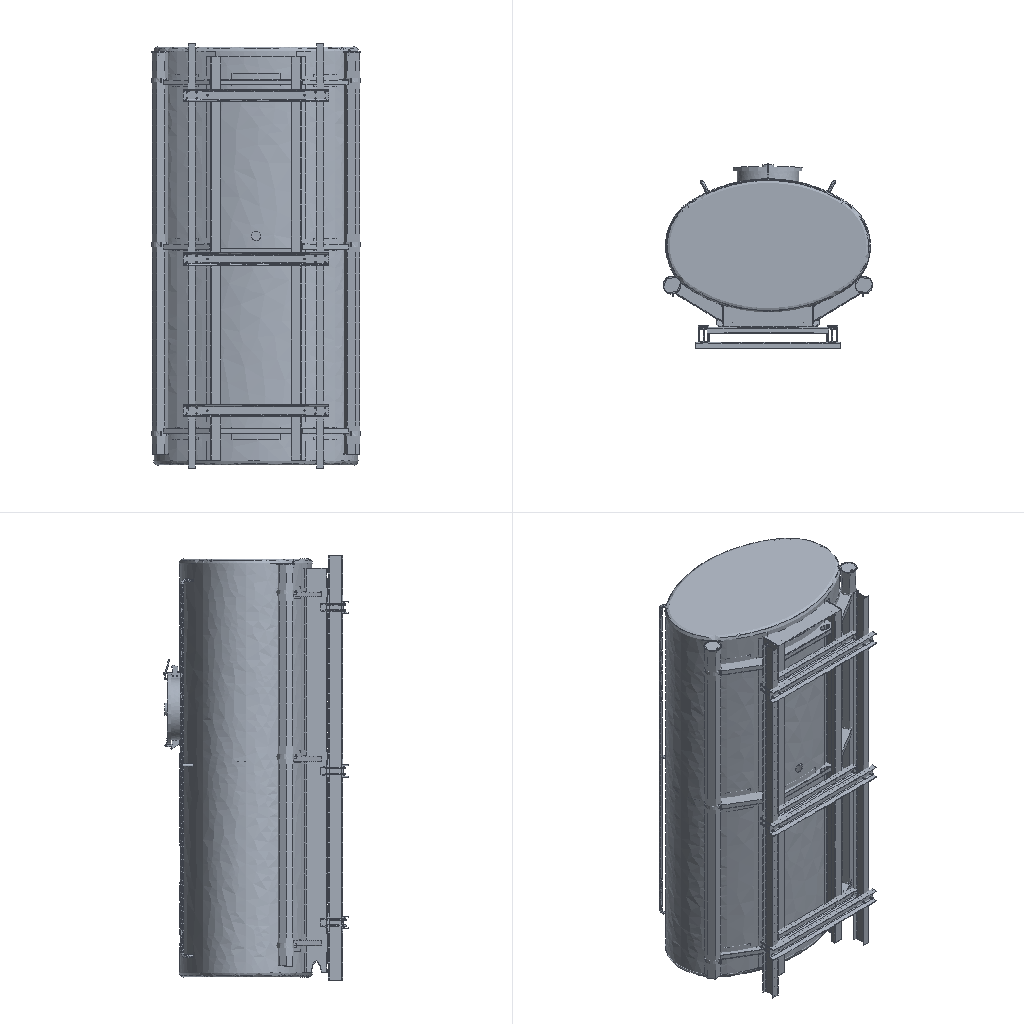Simulation study | ansys workbench
Ansys APDL input file, long lists of numbers shortened:
/batch
/config,noeldb,1     ! force off writing results to database
*get,_wallstrt,active,,time,wall
! ANSYS input file written by Workbench version 2022 R1
! File used for geometry attach: F:\ansys（分析文件汇总)\洒水车有限元分析\晒水车罐体.STEP
/title,wbnew--____ (D5)
! ****** Begin Custom Load Command Snippet ******
/COM, ACT Extensions:
/COM,     LSDYNA, 2021.1
/COM,
! ****** End   Custom Load Command Snippet ******
*DIM,_wb_ProjectScratch_dir,string,248
_wb_ProjectScratch_dir(1) = 'C:\Users\Administrator\AppData\Local\Temp\WB_Administrator_19044_2\_ProjectScratch\ScrCD54\'
*DIM,_wb_SolverFiles_dir,string,248
_wb_SolverFiles_dir(1) = 'C:\Users\Administrator\AppData\Local\Temp\WB_Administrator_19044_2\wbnew_files\dp0\SYS-2\MECH\'
*DIM,_wb_userfiles_dir,string,248
_wb_userfiles_dir(1) = 'C:\Users\Administrator\AppData\Local\Temp\WB_Administrator_19044_2\wbnew_files\user_files\'
/com,--- Data in consistent NMM units. See Solving Units in the help system for more information.
/units,MPA
/nopr
/wb,file,start              !  signify a WB generated input file
/prep7
! Turn off shape checking because checks already performed inside WB mesher.
! See help system for more information.
SHPP,OFF,,NOWARN
/nolist
etcon,set             ! allow ANSYS to choose best KEYOP's for 180x elements, resets any applicable keyopt to MAPDL defaults
/com,*********** Nodes for the whole assembly ***********
nblock,3,,154514
(1i9,3e20.9e3)
    59613    -4.978285790E+02     4.306437121E+02     3.184288870E+01
! (140467 more lines like these left out)
-1
/wb,elem,start            !  set before creation of elements
/com,*********** Elements for Body 1 "__|1210-011-G03|__-__1" ***********
et,1,187
eblock,19,solid,,5134
(19i9)
        1        1        1        1        0        0        0        0       10        0        1     1367     1730     1457     1374     9329     9682     9325     9324
! (10267 more lines like these left out)
-1
/com,*********** Elements for Body 2 "__|1210-011-G03|__-__1[2]" ***********
et,2,187
eblock,19,solid,,5134
(19i9)
        2        2        2        2        0        0        0        0       10        0     5135    12093    12456    12183    12100    20055    20408    20051    20050
! (10267 more lines like these left out)
-1
/com,*********** Elements for Body 3 "__|__-0|__-__3" ***********
et,3,187
eblock,19,solid,,12299
(19i9)
        3        3        3        3        0        0        0        0       10        0    10269    22599    23787    23678    22852    33647    40850    33645    33640
! (24597 more lines like these left out)
-1
/com,*********** Elements for Body 4 "__|1210-041-G03|__-__9" ***********
et,4,187
eblock,19,solid,,1630
(19i9)
        4        4        4        4        0        0        0        0       10        0    22568    46545    47052    46995    46688    47336    49436    47333    47330
! (3259 more lines like these left out)
-1
/com,*********** Elements for Body 5 "__|1210-042-G03|__-__1" ***********
et,5,186
keyo,5,2,1          ! set full integration on SOLID186
eblock,19,solid,,62
(19i9)
        5        5        5        5        0        0        0        0       20        0    24198    50489    50500    50499    50490    50548    50537    50538    50539
! (123 more lines like these left out)
-1
! (74 more sections like these left out)
/wb,elem,end               !  done creating elements
/com,*********** Send User Defined Coordinate System(s) ***********
csys,0
toffst,273.15,  ! Temperature offset from absolute zero
/com,*********** Set Reference Temperature ***********
tref,22.
/wb,mat,start              !  starting to send materials
/com,*********** Send Materials ***********
Temperature = 'TEMP' ! Temperature
MP,DENS,1,7.85e-09,	! tonne mm^-3
MP,ALPX,1,1.2e-05,	! C^-1
MP,C,1,434000000,	! mm^2 s^-2 C^-1
MP,KXX,1,60.5,	! tonne mm s^-3 C^-1
MP,RSVX,1,0.00017,	! ohm mm
MP,EX,1,200000,	! tonne s^-2 mm^-1
MP,NUXY,1,0.3,
MP,MURX,1,10000,
Temperature = 'TEMP' ! Temperature
MP,DENS,2,7.85e-09,	! tonne mm^-3
MP,ALPX,2,1.2e-05,	! C^-1
MP,C,2,434000000,	! mm^2 s^-2 C^-1
MP,KXX,2,60.5,	! tonne mm s^-3 C^-1
MP,RSVX,2,0.00017,	! ohm mm
MP,EX,2,200000,	! tonne s^-2 mm^-1
MP,NUXY,2,0.3,
MP,MURX,2,10000,
Temperature = 'TEMP' ! Temperature
MP,DENS,3,7.85e-09,	! tonne mm^-3
MP,ALPX,3,1.2e-05,	! C^-1
MP,C,3,434000000,	! mm^2 s^-2 C^-1
MP,KXX,3,60.5,	! tonne mm s^-3 C^-1
MP,RSVX,3,0.00017,	! ohm mm
MP,EX,3,200000,	! tonne s^-2 mm^-1
MP,NUXY,3,0.3,
MP,MURX,3,10000,
Temperature = 'TEMP' ! Temperature
MP,DENS,4,7.85e-09,	! tonne mm^-3
MP,ALPX,4,1.2e-05,	! C^-1
MP,C,4,434000000,	! mm^2 s^-2 C^-1
MP,KXX,4,60.5,	! tonne mm s^-3 C^-1
MP,RSVX,4,0.00017,	! ohm mm
MP,EX,4,200000,	! tonne s^-2 mm^-1
MP,NUXY,4,0.3,
MP,MURX,4,10000,
Temperature = 'TEMP' ! Temperature
MP,DENS,5,7.85e-09,	! tonne mm^-3
MP,ALPX,5,1.2e-05,	! C^-1
MP,C,5,434000000,	! mm^2 s^-2 C^-1
MP,KXX,5,60.5,	! tonne mm s^-3 C^-1
MP,RSVX,5,0.00017,	! ohm mm
MP,EX,5,200000,	! tonne s^-2 mm^-1
MP,NUXY,5,0.3,
MP,MURX,5,10000,
Temperature = 'TEMP' ! Temperature
MP,DENS,6,7.85e-09,	! tonne mm^-3
MP,ALPX,6,1.2e-05,	! C^-1
MP,C,6,434000000,	! mm^2 s^-2 C^-1
MP,KXX,6,60.5,	! tonne mm s^-3 C^-1
MP,RSVX,6,0.00017,	! ohm mm
MP,EX,6,200000,	! tonne s^-2 mm^-1
MP,NUXY,6,0.3,
MP,MURX,6,10000,
Temperature = 'TEMP' ! Temperature
MP,DENS,7,7.85e-09,	! tonne mm^-3
MP,ALPX,7,1.2e-05,	! C^-1
MP,C,7,434000000,	! mm^2 s^-2 C^-1
MP,KXX,7,60.5,	! tonne mm s^-3 C^-1
MP,RSVX,7,0.00017,	! ohm mm
MP,EX,7,200000,	! tonne s^-2 mm^-1
MP,NUXY,7,0.3,
MP,MURX,7,10000,
Temperature = 'TEMP' ! Temperature
MP,DENS,8,7.85e-09,	! tonne mm^-3
MP,ALPX,8,1.2e-05,	! C^-1
MP,C,8,434000000,	! mm^2 s^-2 C^-1
MP,KXX,8,60.5,	! tonne mm s^-3 C^-1
MP,RSVX,8,0.00017,	! ohm mm
MP,EX,8,200000,	! tonne s^-2 mm^-1
MP,NUXY,8,0.3,
MP,MURX,8,10000,
Temperature = 'TEMP' ! Temperature
MP,DENS,9,7.85e-09,	! tonne mm^-3
MP,ALPX,9,1.2e-05,	! C^-1
MP,C,9,434000000,	! mm^2 s^-2 C^-1
MP,KXX,9,60.5,	! tonne mm s^-3 C^-1
MP,RSVX,9,0.00017,	! ohm mm
MP,EX,9,200000,	! tonne s^-2 mm^-1
! (632 more lines like these left out)
/wb,mat,end                !  done sending materials
!************************* Model Summary ********************
!__|1210-011-G03|__-__1,	Q235B,	matid,	1
!__|1210-011-G03|__-__1[2],	Q235B,	matid,	2
!__|__-0|__-__3,	Q235B,	matid,	3
! (78 more lines like these left out)
*get,_xmin,node,,mnloc,x
*get,_ymin,node,,mnloc,y
*get,_zmin,node,,mnloc,z
*get,_xmax,node,,mxloc,x
*get,_ymax,node,,mxloc,y
*get,_zmax,node,,mxloc,z
_ASMDIAG=(_xmax-_xmin)*(_xmax-_xmin)+(_ymax-_ymin)*(_ymax-_ymin)+(_zmax-_zmin)*(_zmax-_zmin)
_ASMDIAG=SQRT(_ASMDIAG)
/wb,contact,start          !  starting to send contact
/com,*********** Create Contact "接触区域" ***********
/com,            Real Constant Set For Above Contact Is 81 & 80
*set,tid,81
*set,cid,80
r,tid
r,cid
et,tid,170
et,cid,174
eblock,10,,,316
(15i9)
   106793       81       81       81        0      240      526      550      550     3708     5545      550     3709
! (315 more lines like these left out)
-1
eblock,10,,,316
(15i9)
   107109       80       80       80        0      240      526      550      550     3708     5545      550     3709
! (315 more lines like these left out)
-1
eblock,10,,,119
(15i9)
   107425       80       81       80        0    21474    21805    21997    21997    25860    28558    21997    25861
! (118 more lines like these left out)
-1
eblock,10,,,119
(15i9)
   107544       81       80       81        0    21474    21805    21997    21997    25860    28558    21997    25861
! (118 more lines like these left out)
-1
keyo,cid,8,2               ! auto create asymmetric contact (from Program Controlled setting)
keyo,cid,10,0              ! adjust contact stiffness each NR iteration (from Program Controlled setting)
keyo,cid,12,5              ! bonded always
keyo,cid,18,1              ! small sliding turned on by application
keyo,cid,2,0               ! augmented Lagrange (from Program Controlled setting)
keyo,cid,4,0               ! on Gauss point (from Program Controlled setting)
keyo,cid,9,1               ! ignore initial gaps/penetration
keyo,cid,7,0               ! No Prediction
rmod,tid,3,10.      ! FKN
rmod,tid,5,0.       ! ICONT
rmod,tid,6,0.       ! PINB
rmod,tid,10,0.      ! CNOF
rmod,tid,12,0.      ! FKT
rmod,tid,36,260     ! WB DSID
rmod,cid,3,10.      ! FKN
rmod,cid,5,0.       ! ICONT
rmod,cid,6,0.       ! PINB
rmod,cid,10,0.      ! CNOF
rmod,cid,12,0.      ! FKT
rmod,cid,36,260     ! WB DSID
/com,*********** Create Contact "接触区域 2" ***********
/com,            Real Constant Set For Above Contact Is 83 & 82
*set,tid,83
*set,cid,82
r,tid
r,cid
et,tid,170
et,cid,174
eblock,10,,,10
(15i9)
   107663       83       83       83        0      221      499      516      516     3552     5438      516     3554
! (9 more lines like these left out)
-1
eblock,10,,,10
(15i9)
   107673       82       82       82        0      221      499      516      516     3552     5438      516     3554
! (9 more lines like these left out)
-1
eblock,10,,,2
(15i9)
   107683       82       83       82        0    63922    63923    63749    63747    64830    64280    64275    64276
   107684       82       83       82        0    63923    64008    63748    63749    64835    64279    64277    64280
-1
eblock,10,,,2
(15i9)
   107685       83       82       83        0    63922    63923    63749    63747    64830    64280    64275    64276
   107686       83       82       83        0    63923    64008    63748    63749    64835    64279    64277    64280
-1
keyo,cid,8,2               ! auto create asymmetric contact (from Program Controlled setting)
keyo,cid,10,0              ! adjust contact stiffness each NR iteration (from Program Controlled setting)
keyo,cid,12,5              ! bonded always
keyo,cid,18,1              ! small sliding turned on by application
keyo,cid,2,0               ! augmented Lagrange (from Program Controlled setting)
keyo,cid,4,0               ! on Gauss point (from Program Controlled setting)
keyo,cid,9,1               ! ignore initial gaps/penetration
keyo,cid,7,0               ! No Prediction
rmod,tid,3,10.      ! FKN
rmod,tid,5,0.       ! ICONT
rmod,tid,6,0.       ! PINB
rmod,tid,10,0.      ! CNOF
rmod,tid,12,0.      ! FKT
rmod,tid,36,263     ! WB DSID
rmod,cid,3,10.      ! FKN
rmod,cid,5,0.       ! ICONT
rmod,cid,6,0.       ! PINB
rmod,cid,10,0.      ! CNOF
rmod,cid,12,0.      ! FKT
rmod,cid,36,263     ! WB DSID
/com,*********** Create Contact "接触区域 3" ***********
/com,            Real Constant Set For Above Contact Is 85 & 84
*set,tid,85
*set,cid,84
r,tid
r,cid
et,tid,170
et,cid,174
eblock,10,,,27
(15i9)
   107687       85       85       85        0      221      499      516      516     3552     5438      516     3554
! (26 more lines like these left out)
-1
eblock,10,,,27
(15i9)
   107714       84       84       84        0      221      499      516      516     3552     5438      516     3554
! (26 more lines like these left out)
-1
eblock,10,,,173
(15i9)
   107741       84       85       84        0    65546    65628    65630    65630    65873    66412    65630    65874
! (172 more lines like these left out)
-1
eblock,10,,,173
(15i9)
   107914       85       84       85        0    65546    65628    65630    65630    65873    66412    65630    65874
! (172 more lines like these left out)
-1
keyo,cid,8,2               ! auto create asymmetric contact (from Program Controlled setting)
keyo,cid,10,0              ! adjust contact stiffness each NR iteration (from Program Controlled setting)
keyo,cid,12,5              ! bonded always
keyo,cid,18,1              ! small sliding turned on by application
keyo,cid,2,0               ! augmented Lagrange (from Program Controlled setting)
keyo,cid,4,0               ! on Gauss point (from Program Controlled setting)
keyo,cid,9,1               ! ignore initial gaps/penetration
keyo,cid,7,0               ! No Prediction
rmod,tid,3,10.      ! FKN
rmod,tid,5,0.       ! ICONT
rmod,tid,6,0.       ! PINB
rmod,tid,10,0.      ! CNOF
rmod,tid,12,0.      ! FKT
rmod,tid,36,266     ! WB DSID
rmod,cid,3,10.      ! FKN
rmod,cid,5,0.       ! ICONT
rmod,cid,6,0.       ! PINB
rmod,cid,10,0.      ! CNOF
rmod,cid,12,0.      ! FKT
rmod,cid,36,266     ! WB DSID
/com,*********** Create Contact "接触区域 4" ***********
/com,            Real Constant Set For Above Contact Is 87 & 86
*set,tid,87
*set,cid,86
r,tid
r,cid
et,tid,170
et,cid,174
eblock,10,,,33
(15i9)
   108087       87       87       87        0      303      652      668      668     4185     5810      668     4187
! (32 more lines like these left out)
-1
eblock,10,,,33
(15i9)
   108120       86       86       86        0      303      652      668      668     4185     5810      668     4187
! (32 more lines like these left out)
-1
eblock,10,,,34
(15i9)
   108153       86       87       86        0    68869    68866    68870    68870    69399    69400    68870    69417
! (33 more lines like these left out)
-1
eblock,10,,,34
(15i9)
   108187       87       86       87        0    68869    68866    68870    68870    69399    69400    68870    69417
! (33 more lines like these left out)
-1
keyo,cid,8,2               ! auto create asymmetric contact (from Program Controlled setting)
keyo,cid,10,0              ! adjust contact stiffness each NR iteration (from Program Controlled setting)
keyo,cid,12,5              ! bonded always
keyo,cid,18,1              ! small sliding turned on by application
keyo,cid,2,0               ! augmented Lagrange (from Program Controlled setting)
keyo,cid,4,0               ! on Gauss point (from Program Controlled setting)
keyo,cid,9,1               ! ignore initial gaps/penetration
keyo,cid,7,0               ! No Prediction
rmod,tid,3,10.      ! FKN
rmod,tid,5,0.       ! ICONT
rmod,tid,6,0.       ! PINB
rmod,tid,10,0.      ! CNOF
rmod,tid,12,0.      ! FKT
rmod,tid,36,269     ! WB DSID
rmod,cid,3,10.      ! FKN
rmod,cid,5,0.       ! ICONT
rmod,cid,6,0.       ! PINB
rmod,cid,10,0.      ! CNOF
rmod,cid,12,0.      ! FKT
rmod,cid,36,269     ! WB DSID
/com,*********** Create Contact "接触区域 5" ***********
/com,            Real Constant Set For Above Contact Is 89 & 88
*set,tid,89
*set,cid,88
r,tid
r,cid
et,tid,170
et,cid,174
eblock,10,,,11
(15i9)
   108221       89       89       89        0       42      552      528      528     2210     5551      528     2209
! (10 more lines like these left out)
-1
eblock,10,,,11
(15i9)
   108232       88       88       88        0       42      552      528      528     2210     5551      528     2209
! (10 more lines like these left out)
-1
eblock,10,,,1
(15i9)
   108243       88       89       88        0    84030    84031    84032    84033    84160    84162    84163    84161
-1
eblock,10,,,1
(15i9)
   108244       89       88       89        0    84030    84031    84032    84033    84160    84162    84163    84161
-1
keyo,cid,8,2               ! auto create asymmetric contact (from Program Controlled setting)
keyo,cid,10,0              ! adjust contact stiffness each NR iteration (from Program Controlled setting)
keyo,cid,12,5              ! bonded always
keyo,cid,18,1              ! small sliding turned on by application
keyo,cid,2,0               ! augmented Lagrange (from Program Controlled setting)
keyo,cid,4,0               ! on Gauss point (from Program Controlled setting)
keyo,cid,9,1               ! ignore initial gaps/penetration
keyo,cid,7,0               ! No Prediction
rmod,tid,3,10.      ! FKN
rmod,tid,5,0.       ! ICONT
rmod,tid,6,0.       ! PINB
rmod,tid,10,0.      ! CNOF
rmod,tid,12,0.      ! FKT
rmod,tid,36,272     ! WB DSID
rmod,cid,3,10.      ! FKN
rmod,cid,5,0.       ! ICONT
rmod,cid,6,0.       ! PINB
rmod,cid,10,0.      ! CNOF
rmod,cid,12,0.      ! FKT
rmod,cid,36,272     ! WB DSID
! (211 more sections like these left out)
/wb,contact,end            !  done creating contacts
/golist
/wb,load,start             !  starting to send loads
/com,*********** Fixed Supports ***********
CMBLOCK,_FIXEDSU,NODE,    81922
(8i10)
        19        21        22        23        96        97        98        99
! (10240 more lines like these left out)
cmsel,s,_FIXEDSU
d,all,all
nsel,all
/com,*********** Define Pressure Using Surface Effect Elements "__" ***********
et,512,154
eblock,10,,,2197
(15i9)
   141235      512      512      512        0    25694    22771    25685    25685    35439    35437    25685    46526
! (2196 more lines like these left out)
-1
esel,s,type,,512
keyop,512,7,0                ! Use deformed area for application of load
esel,all
esel,all
/gst,on,on
fini
*get,_numnode,node,0,count
*get,_numelem,elem,0,count
*get, _MAXELEMNUM, elem, 0, NUM, MAX
*get, _MAXNODENUM, node, 0, NUM, MAX
*get, _MAXELEMTYPE, etyp, 0, NUM, MAX
*get, _MAXREALCONST, real, 0, NUM, MAX
/go
/wb,load,end               !  done creating loads
/com,--- Number of total nodes = %_numnode%
/com,--- Number of contact elements = 36639
/com,--- Number of spring elements = 0
/com,--- Number of bearing elements = 0
/com,--- Number of solid elements = 58082
/com,--- Number of condensed parts = 0
/com,--- Number of total elements = %_numelem%
*get,_wallbsol,active,,time,wall
/com,****************************************************************************
/com,*************************    SOLUTION       ********************************
/com,****************************************************************************
/solu
antype,0                   ! static analysis
_thickRatio=  0     ! Ratio of thick parts in the model
eqsl,sparse,,,,,1
cntr,print,1               ! print out contact info and also make no initial contact an error
cntr,out,yes               ! write contact output to file.cmn due to many contact pairs present
dmpoption,emat,no             ! Don't combine emat file for DANSYS
dmpoption,esav,no             ! Don't combine esav file for DANSYS
nldiag,cont,iter           ! print out contact info each equilibrium iteration
rescontrol,,none                 ! Do not keep any restart files
/com,****************************************************
/com,******************* SOLVE FOR LS 1 OF 1 ****************
esel,s,type,,512
nsle
sf,all,pres,0.6
nsel,all
esel,all
esel,all
/nopr
/gopr
nsub,1,1,1
time,1.
outres,erase
outres,all,none
outres,nsol,all,
outres,rsol,all
outres,eangl,all
outres,etmp,all
outres,veng,all
outres,strs,all,
outres,epel,all,
outres,eppl,all,
outres,cont,all,
! *********** WB SOLVE COMMAND ***********
! check interactive state
*get,ANSINTER_,active,,int
*if,ANSINTER_,ne,0,then
/eof
*endif
solve
/com *************** Write FE CONNECTORS *********
CEWRITE,file,ce,,INTE
/com,****************************************************
/com,*************** FINISHED SOLVE FOR LS 1 *************
*get,_wallasol,active,,time,wall
/nopr
*get,_numnode,node,0,count
*get,_numelem,elem,0,count
*get, _MAXELEMNUM, elem, 0, NUM, MAX
*get, _MAXNODENUM, node, 0, NUM, MAX,,,INTERNAL
*get, _MAXELEMTYPE, etyp, 0, NUM, MAX
*get, _MAXREALCONST, real, 0, NUM, MAX
/gopr
/post1
xmlo,ENCODING,ISO-8859-1
xmlo,parm
/xml,parm,xml
fini
/gopr
*get,_walldone,active,,time,wall
_preptime=(_wallbsol-_wallstrt)*3600
_solvtime=(_wallasol-_wallbsol)*3600
_posttime=(_walldone-_wallasol)*3600
_totaltim=(_walldone-_wallstrt)*3600
*get,_dlbratio,active,0,solu,dlbr
*get,_combtime,active,0,solu,comb
*get,_ssmode,active,0,solu,ssmm
*get,_ndofs,active,0,solu,ndof
*get,_sol_end_time,active,0,set,time
*if,_sol_end_time,eq,1.,then
/fclean				!clean distributed files
*endif
/com,--- Total number of nodes = %_numnode%
/com,--- Total number of elements = %_numelem%
/com,--- Element load balance ratio = %_dlbratio%
/com,--- Time to combine distributed files = %_combtime%
/com,--- Sparse memory mode = %_ssmode%
/com,--- Number of DOF = %_ndofs%
/wb,file,end               ! done with WB generated input